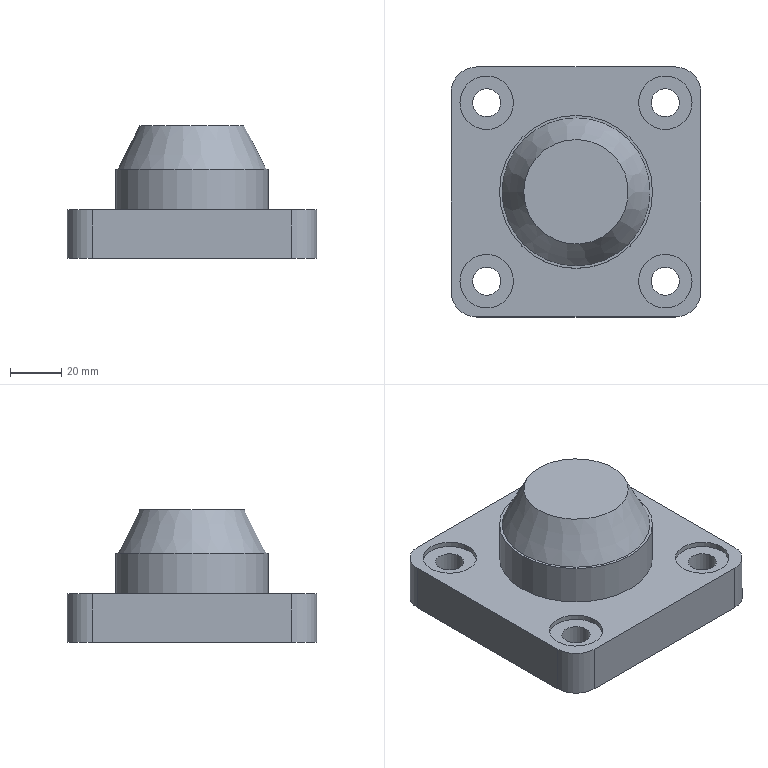Part | STEP file | 50502A | 1 solid | 32 faces | box 98 x 98 x 52 mm | volume 215908 mm3 | spline 12 | plane 11 | cylinder 8 | cone 1 | commonest cylinder face diameters 20 x4 25 x1 35 x1 58 x1 60 x1